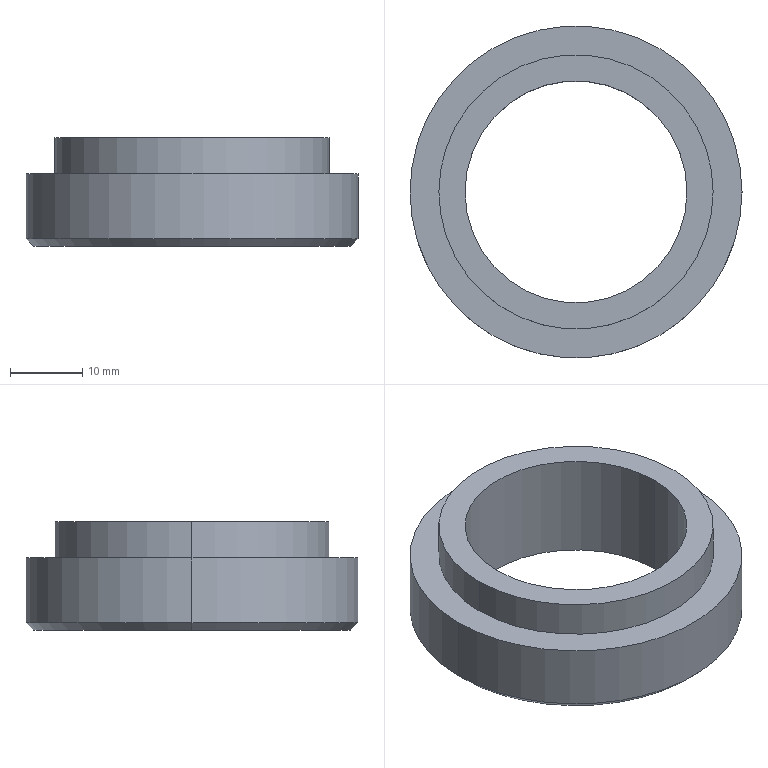Part | SolidWorks | features ICE 3, Chamfer 1, Extrusion 1, HoleWzd 1 | 1 solid | 11 faces | box 46 x 46 x 15 mm | volume 11079 mm3 | cylinder 6 | plane 3 | cone 2 | commonest cylinder face diameters 30.75 x2 38 x2 46 x2
STEP:
#1=CARTESIAN_POINT('',(-22.,0.,10.));
#2=VERTEX_POINT('',#1);
#3=CARTESIAN_POINT('',(22.,0.,10.));
#4=VERTEX_POINT('',#3);
#5=CARTESIAN_POINT('',(0.,0.,10.));
#6=DIRECTION('',(0.,0.,-1.));
#7=DIRECTION('',(1.,0.,0.));
#8=AXIS2_PLACEMENT_3D('',#5,#6,#7);
#9=CIRCLE('',#8,22.);
#10=EDGE_CURVE('',#2,#4,#9,.T.);
#11=ORIENTED_EDGE('',*,*,#10,.F.);
#12=CARTESIAN_POINT('',(-23.,0.,11.));
#13=VERTEX_POINT('',#12);
#14=CARTESIAN_POINT('',(-23.,0.,11.));
#15=DIRECTION('',(-0.7071,0.,0.7071));
#16=VECTOR('',#15,1000.);
#17=LINE('',#14,#16);
#18=EDGE_CURVE('',#2,#13,#17,.T.);
#19=ORIENTED_EDGE('',*,*,#18,.T.);
#20=CARTESIAN_POINT('',(23.,0.,11.));
#21=VERTEX_POINT('',#20);
#22=CARTESIAN_POINT('',(0.,0.,11.));
#23=DIRECTION('',(0.,0.,1.));
#24=DIRECTION('',(1.,0.,0.));
#25=AXIS2_PLACEMENT_3D('',#22,#23,#24);
#26=CIRCLE('',#25,23.);
#27=EDGE_CURVE('',#21,#13,#26,.T.);
#28=ORIENTED_EDGE('',*,*,#27,.F.);
#29=CARTESIAN_POINT('',(23.,0.,11.));
#30=DIRECTION('',(0.7071,0.,0.7071));
#31=VECTOR('',#30,1000.);
#32=LINE('',#29,#31);
#33=EDGE_CURVE('',#4,#21,#32,.T.);
#34=ORIENTED_EDGE('',*,*,#33,.F.);
#35=EDGE_LOOP('',(#11,#19,#28,#34));
#36=FACE_OUTER_BOUND('',#35,.T.);
#37=CARTESIAN_POINT('',(0.,0.,11.));
#38=DIRECTION('',(0.,0.,1.));
#39=DIRECTION('',(1.,0.,0.));
#40=AXIS2_PLACEMENT_3D('',#37,#38,#39);
#41=CONICAL_SURFACE('',#40,23.,0.7854);
#42=ADVANCED_FACE('',(#36),#41,.T.);
#43=CARTESIAN_POINT('',(15.375,0.,10.));
#44=VERTEX_POINT('',#43);
#45=CARTESIAN_POINT('',(-15.375,0.,10.));
#46=VERTEX_POINT('',#45);
#47=CARTESIAN_POINT('',(0.,0.,10.));
#48=DIRECTION('',(0.,0.,-1.));
#49=DIRECTION('',(1.,0.,0.));
#50=AXIS2_PLACEMENT_3D('',#47,#48,#49);
#51=CIRCLE('',#50,15.375);
#52=EDGE_CURVE('',#44,#46,#51,.T.);
#53=ORIENTED_EDGE('',*,*,#52,.T.);
#54=CARTESIAN_POINT('',(-15.375,0.,25.));
#55=VERTEX_POINT('',#54);
#56=CARTESIAN_POINT('',(-15.375,0.,25.));
#57=DIRECTION('',(0.,0.,1.));
#58=VECTOR('',#57,1000.);
#59=LINE('',#56,#58);
#60=EDGE_CURVE('',#46,#55,#59,.T.);
#61=ORIENTED_EDGE('',*,*,#60,.T.);
#62=CARTESIAN_POINT('',(15.375,0.,25.));
#63=VERTEX_POINT('',#62);
#64=CARTESIAN_POINT('',(0.,0.,25.));
#65=DIRECTION('',(0.,0.,1.));
#66=DIRECTION('',(1.,0.,0.));
#67=AXIS2_PLACEMENT_3D('',#64,#65,#66);
#68=CIRCLE('',#67,15.375);
#69=EDGE_CURVE('',#55,#63,#68,.T.);
#70=ORIENTED_EDGE('',*,*,#69,.T.);
#71=CARTESIAN_POINT('',(15.375,0.,25.));
#72=DIRECTION('',(0.,0.,1.));
#73=VECTOR('',#72,1000.);
#74=LINE('',#71,#73);
#75=EDGE_CURVE('',#44,#63,#74,.T.);
#76=ORIENTED_EDGE('',*,*,#75,.F.);
#77=EDGE_LOOP('',(#53,#61,#70,#76));
#78=FACE_OUTER_BOUND('',#77,.T.);
#79=CARTESIAN_POINT('',(0.,0.,25.));
#80=DIRECTION('',(0.,0.,1.));
#81=DIRECTION('',(1.,0.,0.));
#82=AXIS2_PLACEMENT_3D('',#79,#80,#81);
#83=CYLINDRICAL_SURFACE('',#82,15.375);
#84=ADVANCED_FACE('',(#78),#83,.F.);
#85=CARTESIAN_POINT('',(19.,0.,25.));
#86=VERTEX_POINT('',#85);
#87=CARTESIAN_POINT('',(-19.,0.,25.));
#88=VERTEX_POINT('',#87);
#89=CARTESIAN_POINT('',(0.,0.,25.));
#90=DIRECTION('',(0.,0.,1.));
#91=DIRECTION('',(1.,0.,0.));
#92=AXIS2_PLACEMENT_3D('',#89,#90,#91);
#93=CIRCLE('',#92,19.);
#94=EDGE_CURVE('',#86,#88,#93,.T.);
#95=ORIENTED_EDGE('',*,*,#94,.F.);
#96=CARTESIAN_POINT('',(19.,0.,20.));
#97=VERTEX_POINT('',#96);
#98=CARTESIAN_POINT('',(19.,0.,25.));
#99=DIRECTION('',(0.,0.,-1.));
#100=VECTOR('',#99,1000.);
#101=LINE('',#98,#100);
#102=EDGE_CURVE('',#86,#97,#101,.T.);
#103=ORIENTED_EDGE('',*,*,#102,.T.);
#104=CARTESIAN_POINT('',(-19.,0.,20.));
#105=VERTEX_POINT('',#104);
#106=CARTESIAN_POINT('',(0.,0.,20.));
#107=DIRECTION('',(0.,0.,1.));
#108=DIRECTION('',(1.,0.,0.));
#109=AXIS2_PLACEMENT_3D('',#106,#107,#108);
#110=CIRCLE('',#109,19.);
#111=EDGE_CURVE('',#97,#105,#110,.T.);
#112=ORIENTED_EDGE('',*,*,#111,.T.);
#113=CARTESIAN_POINT('',(-19.,0.,25.));
#114=DIRECTION('',(0.,0.,-1.));
#115=VECTOR('',#114,1000.);
#116=LINE('',#113,#115);
#117=EDGE_CURVE('',#88,#105,#116,.T.);
#118=ORIENTED_EDGE('',*,*,#117,.F.);
#119=EDGE_LOOP('',(#95,#103,#112,#118));
#120=FACE_OUTER_BOUND('',#119,.T.);
#121=CARTESIAN_POINT('',(0.,0.,25.));
#122=DIRECTION('',(0.,0.,-1.));
#123=DIRECTION('',(-1.,0.,0.));
#124=AXIS2_PLACEMENT_3D('',#121,#122,#123);
#125=CYLINDRICAL_SURFACE('',#124,19.);
#126=ADVANCED_FACE('',(#120),#125,.T.);
#127=CARTESIAN_POINT('',(23.,0.,20.));
#128=VERTEX_POINT('',#127);
#129=CARTESIAN_POINT('',(-23.,0.,20.));
#130=VERTEX_POINT('',#129);
#131=CARTESIAN_POINT('',(0.,0.,20.));
#132=DIRECTION('',(0.,0.,1.));
#133=DIRECTION('',(1.,0.,0.));
#134=AXIS2_PLACEMENT_3D('',#131,#132,#133);
#135=CIRCLE('',#134,23.);
#136=EDGE_CURVE('',#128,#130,#135,.T.);
#137=ORIENTED_EDGE('',*,*,#136,.F.);
#138=CARTESIAN_POINT('',(23.,0.,20.));
#139=DIRECTION('',(0.,0.,-1.));
#140=VECTOR('',#139,1000.);
#141=LINE('',#138,#140);
#142=EDGE_CURVE('',#128,#21,#141,.T.);
#143=ORIENTED_EDGE('',*,*,#142,.T.);
#144=ORIENTED_EDGE('',*,*,#27,.T.);
#145=CARTESIAN_POINT('',(-23.,0.,20.));
#146=DIRECTION('',(0.,0.,-1.));
#147=VECTOR('',#146,1000.);
#148=LINE('',#145,#147);
#149=EDGE_CURVE('',#130,#13,#148,.T.);
#150=ORIENTED_EDGE('',*,*,#149,.F.);
#151=EDGE_LOOP('',(#137,#143,#144,#150));
#152=FACE_OUTER_BOUND('',#151,.T.);
#153=CARTESIAN_POINT('',(0.,0.,20.));
#154=DIRECTION('',(0.,0.,-1.));
#155=DIRECTION('',(-1.,0.,0.));
#156=AXIS2_PLACEMENT_3D('',#153,#154,#155);
#157=CYLINDRICAL_SURFACE('',#156,23.);
#158=ADVANCED_FACE('',(#152),#157,.T.);
#159=CARTESIAN_POINT('',(0.,0.,20.));
#160=DIRECTION('',(0.,0.,1.));
#161=DIRECTION('',(1.,0.,0.));
#162=AXIS2_PLACEMENT_3D('',#159,#160,#161);
#163=CIRCLE('',#162,19.);
#164=EDGE_CURVE('',#105,#97,#163,.T.);
#165=ORIENTED_EDGE('',*,*,#164,.F.);
#166=ORIENTED_EDGE('',*,*,#111,.F.);
#167=EDGE_LOOP('',(#165,#166));
#168=FACE_BOUND('',#167,.T.);
#169=CARTESIAN_POINT('',(0.,0.,20.));
#170=DIRECTION('',(0.,0.,1.));
#171=DIRECTION('',(1.,0.,0.));
#172=AXIS2_PLACEMENT_3D('',#169,#170,#171);
#173=CIRCLE('',#172,23.);
#174=EDGE_CURVE('',#130,#128,#173,.T.);
#175=ORIENTED_EDGE('',*,*,#174,.T.);
#176=ORIENTED_EDGE('',*,*,#136,.T.);
#177=EDGE_LOOP('',(#175,#176));
#178=FACE_OUTER_BOUND('',#177,.T.);
#179=CARTESIAN_POINT('',(0.,0.,20.));
#180=DIRECTION('',(0.,0.,1.));
#181=DIRECTION('',(1.,0.,0.));
#182=AXIS2_PLACEMENT_3D('',#179,#180,#181);
#183=PLANE('',#182);
#184=ADVANCED_FACE('',(#168,#178),#183,.T.);
#185=CARTESIAN_POINT('',(0.,0.,10.));
#186=DIRECTION('',(0.,0.,-1.));
#187=DIRECTION('',(1.,0.,0.));
#188=AXIS2_PLACEMENT_3D('',#185,#186,#187);
#189=CIRCLE('',#188,22.);
#190=EDGE_CURVE('',#4,#2,#189,.T.);
#191=ORIENTED_EDGE('',*,*,#190,.T.);
#192=ORIENTED_EDGE('',*,*,#10,.T.);
#193=EDGE_LOOP('',(#191,#192));
#194=FACE_OUTER_BOUND('',#193,.T.);
#195=ORIENTED_EDGE('',*,*,#52,.F.);
#196=CARTESIAN_POINT('',(0.,0.,10.));
#197=DIRECTION('',(0.,0.,-1.));
#198=DIRECTION('',(1.,0.,0.));
#199=AXIS2_PLACEMENT_3D('',#196,#197,#198);
#200=CIRCLE('',#199,15.375);
#201=EDGE_CURVE('',#46,#44,#200,.T.);
#202=ORIENTED_EDGE('',*,*,#201,.F.);
#203=EDGE_LOOP('',(#195,#202));
#204=FACE_BOUND('',#203,.T.);
#205=CARTESIAN_POINT('',(0.,0.,10.));
#206=DIRECTION('',(0.,0.,1.));
#207=DIRECTION('',(1.,0.,0.));
#208=AXIS2_PLACEMENT_3D('',#205,#206,#207);
#209=PLANE('',#208);
#210=ADVANCED_FACE('',(#194,#204),#209,.F.);
#211=ORIENTED_EDGE('',*,*,#142,.F.);
#212=ORIENTED_EDGE('',*,*,#174,.F.);
#213=ORIENTED_EDGE('',*,*,#149,.T.);
#214=CARTESIAN_POINT('',(0.,0.,11.));
#215=DIRECTION('',(0.,0.,1.));
#216=DIRECTION('',(1.,0.,0.));
#217=AXIS2_PLACEMENT_3D('',#214,#215,#216);
#218=CIRCLE('',#217,23.);
#219=EDGE_CURVE('',#13,#21,#218,.T.);
#220=ORIENTED_EDGE('',*,*,#219,.T.);
#221=EDGE_LOOP('',(#211,#212,#213,#220));
#222=FACE_OUTER_BOUND('',#221,.T.);
#223=CARTESIAN_POINT('',(0.,0.,20.));
#224=DIRECTION('',(0.,0.,-1.));
#225=DIRECTION('',(-1.,0.,0.));
#226=AXIS2_PLACEMENT_3D('',#223,#224,#225);
#227=CYLINDRICAL_SURFACE('',#226,23.);
#228=ADVANCED_FACE('',(#222),#227,.T.);
#229=CARTESIAN_POINT('',(0.,0.,25.));
#230=DIRECTION('',(0.,0.,1.));
#231=DIRECTION('',(1.,0.,0.));
#232=AXIS2_PLACEMENT_3D('',#229,#230,#231);
#233=CIRCLE('',#232,15.375);
#234=EDGE_CURVE('',#63,#55,#233,.T.);
#235=ORIENTED_EDGE('',*,*,#234,.F.);
#236=ORIENTED_EDGE('',*,*,#69,.F.);
#237=EDGE_LOOP('',(#235,#236));
#238=FACE_BOUND('',#237,.T.);
#239=CARTESIAN_POINT('',(0.,0.,25.));
#240=DIRECTION('',(0.,0.,1.));
#241=DIRECTION('',(1.,0.,0.));
#242=AXIS2_PLACEMENT_3D('',#239,#240,#241);
#243=CIRCLE('',#242,19.);
#244=EDGE_CURVE('',#88,#86,#243,.T.);
#245=ORIENTED_EDGE('',*,*,#244,.T.);
#246=ORIENTED_EDGE('',*,*,#94,.T.);
#247=EDGE_LOOP('',(#245,#246));
#248=FACE_OUTER_BOUND('',#247,.T.);
#249=CARTESIAN_POINT('',(0.,0.,25.));
#250=DIRECTION('',(0.,0.,1.));
#251=DIRECTION('',(1.,0.,0.));
#252=AXIS2_PLACEMENT_3D('',#249,#250,#251);
#253=PLANE('',#252);
#254=ADVANCED_FACE('',(#238,#248),#253,.T.);
#255=ORIENTED_EDGE('',*,*,#102,.F.);
#256=ORIENTED_EDGE('',*,*,#244,.F.);
#257=ORIENTED_EDGE('',*,*,#117,.T.);
#258=ORIENTED_EDGE('',*,*,#164,.T.);
#259=EDGE_LOOP('',(#255,#256,#257,#258));
#260=FACE_OUTER_BOUND('',#259,.T.);
#261=CARTESIAN_POINT('',(0.,0.,25.));
#262=DIRECTION('',(0.,0.,-1.));
#263=DIRECTION('',(-1.,0.,0.));
#264=AXIS2_PLACEMENT_3D('',#261,#262,#263);
#265=CYLINDRICAL_SURFACE('',#264,19.);
#266=ADVANCED_FACE('',(#260),#265,.T.);
#267=ORIENTED_EDGE('',*,*,#60,.F.);
#268=ORIENTED_EDGE('',*,*,#201,.T.);
#269=ORIENTED_EDGE('',*,*,#75,.T.);
#270=ORIENTED_EDGE('',*,*,#234,.T.);
#271=EDGE_LOOP('',(#267,#268,#269,#270));
#272=FACE_OUTER_BOUND('',#271,.T.);
#273=CARTESIAN_POINT('',(0.,0.,25.));
#274=DIRECTION('',(0.,0.,1.));
#275=DIRECTION('',(1.,0.,0.));
#276=AXIS2_PLACEMENT_3D('',#273,#274,#275);
#277=CYLINDRICAL_SURFACE('',#276,15.375);
#278=ADVANCED_FACE('',(#272),#277,.F.);
#279=ORIENTED_EDGE('',*,*,#18,.F.);
#280=ORIENTED_EDGE('',*,*,#190,.F.);
#281=ORIENTED_EDGE('',*,*,#33,.T.);
#282=ORIENTED_EDGE('',*,*,#219,.F.);
#283=EDGE_LOOP('',(#279,#280,#281,#282));
#284=FACE_OUTER_BOUND('',#283,.T.);
#285=CARTESIAN_POINT('',(0.,0.,11.));
#286=DIRECTION('',(0.,0.,1.));
#287=DIRECTION('',(1.,0.,0.));
#288=AXIS2_PLACEMENT_3D('',#285,#286,#287);
#289=CONICAL_SURFACE('',#288,23.,0.7854);
#290=ADVANCED_FACE('',(#284),#289,.T.);
#291=CLOSED_SHELL('',(#42,#84,#126,#158,#184,#210,#228,#254,#266,#278,#290));
#292=MANIFOLD_SOLID_BREP('',#291);
#293=CARTESIAN_POINT('',(0.,0.,0.));
#294=DIRECTION('',(0.,0.,1.));
#295=DIRECTION('',(1.,0.,0.));
#296=AXIS2_PLACEMENT_3D('',#293,#294,#295);
#297=(LENGTH_UNIT()NAMED_UNIT(*)SI_UNIT(.MILLI.,.METRE.));
#298=UNCERTAINTY_MEASURE_WITH_UNIT(LENGTH_MEASURE(0.00001),#297,'','');
#299=(NAMED_UNIT(*)PLANE_ANGLE_UNIT()SI_UNIT($,.RADIAN.));
#300=(NAMED_UNIT(*)SI_UNIT($,.STERADIAN.)SOLID_ANGLE_UNIT());
#301=(GEOMETRIC_REPRESENTATION_CONTEXT(3)GLOBAL_UNCERTAINTY_ASSIGNED_CONTEXT((#298))GLOBAL_UNIT_ASSIGNED_CONTEXT((#297,#299,#300))REPRESENTATION_CONTEXT('',''));
#302=ADVANCED_BREP_SHAPE_REPRESENTATION('',(#292,#296),#301);